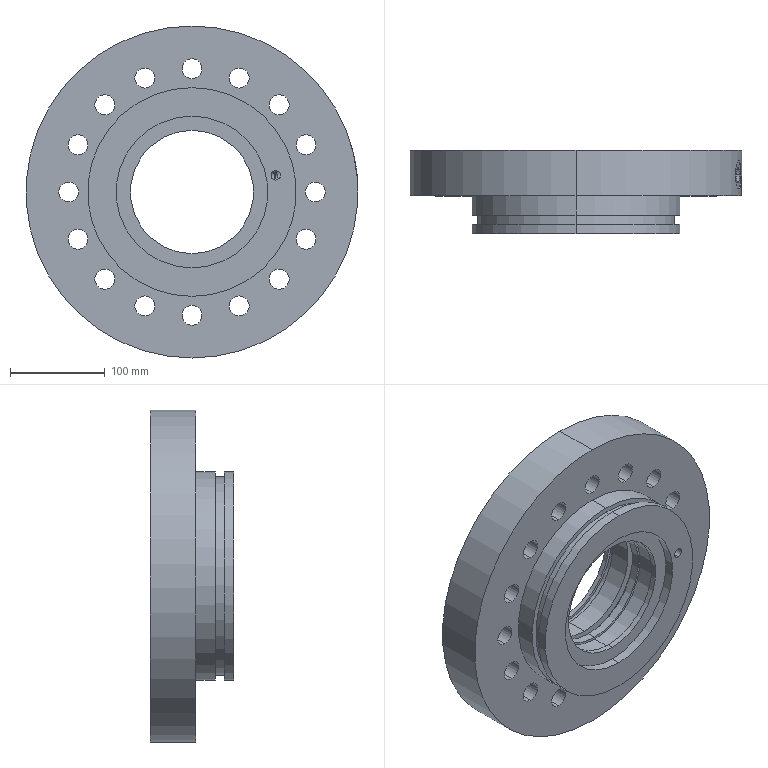Part | SolidWorks | features HoleWzd 4, 3DProfileFeature 1, RefAxis 1, Revolution 1 | 1 solid | 137 faces | box 350 x 88 x 350 mm | volume 4363937 mm3 | cylinder 102 | plane 29 | cone 6 | commonest cylinder face diameters 21 x32 32 x32 10 x10 130 x6 220 x4 16.5 x2